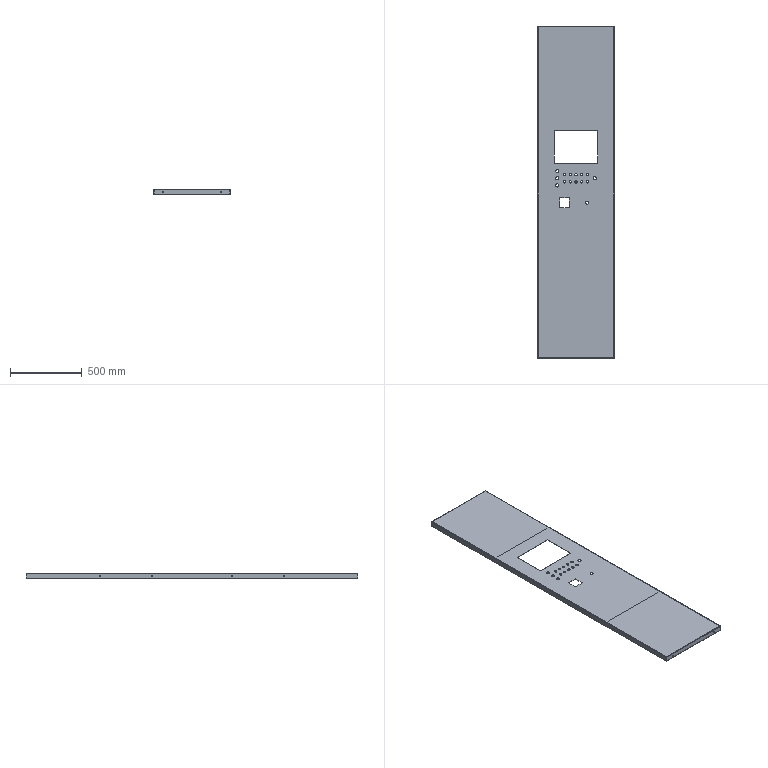Part | SolidWorks | features SMWeldBead 4, EdgeFlange 2, HoleWzd 2, BossThin 1, FlatPattern 1, ICE 1, SMBaseFlange 1, SheetMetal 1 | 1 solid | 187 faces | box 533 x 2311 x 38 mm | volume 2271037 mm3 | cylinder 74 | plane 73 | spline 40 | commonest cylinder face diameters 6.6 x24 16.2 x20 22 x10 4 x8 7 x8 2 x4